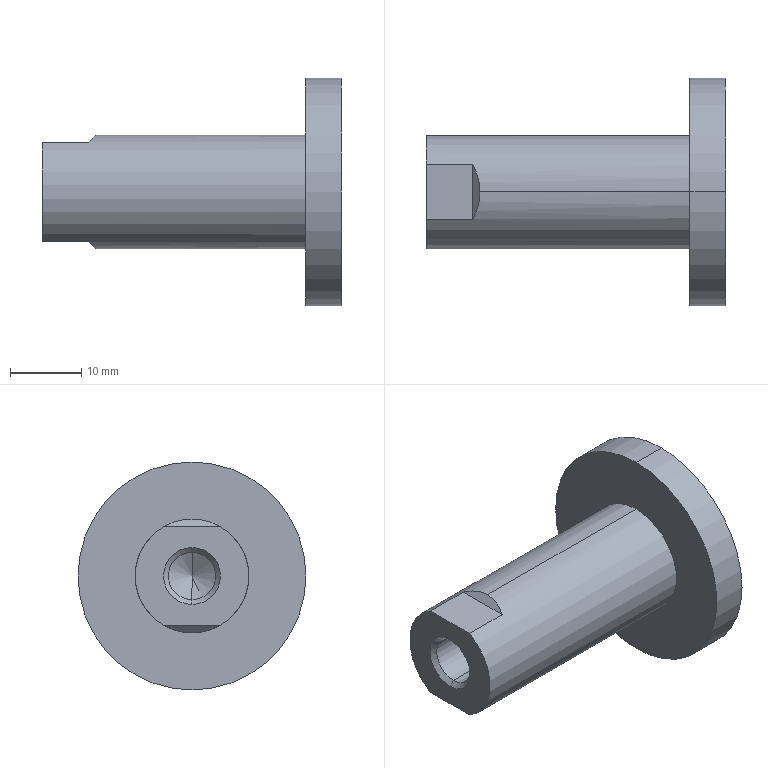Part | SolidWorks | features RefAxis 3, 3DProfileFeature 1, ICE 1, Revolution 1 | 1 solid | 17 faces | box 42 x 32 x 32 mm | volume 10910 mm3 | plane 7 | cylinder 6 | cone 4 | commonest cylinder face diameters 6.647 x2 16 x2 32 x2
STEP:
#1=CARTESIAN_POINT('',(35.,0.,16.));
#2=VERTEX_POINT('',#1);
#3=CARTESIAN_POINT('',(35.,0.,-16.));
#4=VERTEX_POINT('',#3);
#5=CARTESIAN_POINT('',(35.,0.,0.));
#6=DIRECTION('',(-1.,0.,0.));
#7=DIRECTION('',(0.,0.,1.));
#8=AXIS2_PLACEMENT_3D('',#5,#6,#7);
#9=CIRCLE('',#8,16.);
#10=EDGE_CURVE('',#2,#4,#9,.T.);
#11=ORIENTED_EDGE('',*,*,#10,.T.);
#12=CARTESIAN_POINT('',(30.,0.,-16.));
#13=VERTEX_POINT('',#12);
#14=CARTESIAN_POINT('',(35.,0.,-16.));
#15=DIRECTION('',(-1.,0.,0.));
#16=VECTOR('',#15,1000.);
#17=LINE('',#14,#16);
#18=EDGE_CURVE('',#4,#13,#17,.T.);
#19=ORIENTED_EDGE('',*,*,#18,.T.);
#20=CARTESIAN_POINT('',(30.,0.,16.));
#21=VERTEX_POINT('',#20);
#22=CARTESIAN_POINT('',(30.,0.,0.));
#23=DIRECTION('',(-1.,0.,0.));
#24=DIRECTION('',(0.,0.,1.));
#25=AXIS2_PLACEMENT_3D('',#22,#23,#24);
#26=CIRCLE('',#25,16.);
#27=EDGE_CURVE('',#21,#13,#26,.T.);
#28=ORIENTED_EDGE('',*,*,#27,.F.);
#29=CARTESIAN_POINT('',(35.,0.,16.));
#30=DIRECTION('',(-1.,0.,0.));
#31=VECTOR('',#30,1000.);
#32=LINE('',#29,#31);
#33=EDGE_CURVE('',#2,#21,#32,.T.);
#34=ORIENTED_EDGE('',*,*,#33,.F.);
#35=EDGE_LOOP('',(#11,#19,#28,#34));
#36=FACE_OUTER_BOUND('',#35,.T.);
#37=CARTESIAN_POINT('',(35.,0.,0.));
#38=DIRECTION('',(-1.,0.,0.));
#39=DIRECTION('',(0.,0.,1.));
#40=AXIS2_PLACEMENT_3D('',#37,#38,#39);
#41=CYLINDRICAL_SURFACE('',#40,16.);
#42=ADVANCED_FACE('',(#36),#41,.T.);
#43=CARTESIAN_POINT('',(30.,0.,8.));
#44=VERTEX_POINT('',#43);
#45=CARTESIAN_POINT('',(30.,0.,-8.));
#46=VERTEX_POINT('',#45);
#47=CARTESIAN_POINT('',(30.,0.,0.));
#48=DIRECTION('',(-1.,0.,0.));
#49=DIRECTION('',(0.,0.,1.));
#50=AXIS2_PLACEMENT_3D('',#47,#48,#49);
#51=CIRCLE('',#50,8.);
#52=EDGE_CURVE('',#44,#46,#51,.T.);
#53=ORIENTED_EDGE('',*,*,#52,.T.);
#54=CARTESIAN_POINT('',(0.5,0.,-8.));
#55=VERTEX_POINT('',#54);
#56=CARTESIAN_POINT('',(35.,0.,-8.));
#57=DIRECTION('',(-1.,0.,0.));
#58=VECTOR('',#57,1000.);
#59=LINE('',#56,#58);
#60=EDGE_CURVE('',#46,#55,#59,.T.);
#61=ORIENTED_EDGE('',*,*,#60,.T.);
#62=CARTESIAN_POINT('',(-0.5,3.873,-7.));
#63=VERTEX_POINT('',#62);
#64=CARTESIAN_POINT('',(0.5,0.,-8.));
#65=CARTESIAN_POINT('',(0.5,1.362,-8.));
#66=CARTESIAN_POINT('',(0.1595,2.681,-7.659));
#67=CARTESIAN_POINT('',(-0.5,3.873,-7.));
#68=(BOUNDED_CURVE()B_SPLINE_CURVE(3,(#64,#65,#66,#67),.UNSPECIFIED.,.F.,.F.)B_SPLINE_CURVE_WITH_KNOTS((4,4),(3.142,3.647),.UNSPECIFIED.)CURVE()GEOMETRIC_REPRESENTATION_ITEM()RATIONAL_B_SPLINE_CURVE((1.,0.9788,0.9788,1.))REPRESENTATION_ITEM(''));
#69=EDGE_CURVE('',#55,#63,#68,.T.);
#70=ORIENTED_EDGE('',*,*,#69,.T.);
#71=CARTESIAN_POINT('',(-7.,3.873,-7.));
#72=VERTEX_POINT('',#71);
#73=CARTESIAN_POINT('',(35.,3.873,-7.));
#74=DIRECTION('',(-1.,0.,0.));
#75=VECTOR('',#74,1000.);
#76=LINE('',#73,#75);
#77=EDGE_CURVE('',#63,#72,#76,.T.);
#78=ORIENTED_EDGE('',*,*,#77,.T.);
#79=CARTESIAN_POINT('',(-7.,3.873,7.));
#80=VERTEX_POINT('',#79);
#81=CARTESIAN_POINT('',(-7.,0.,0.));
#82=DIRECTION('',(-1.,0.,0.));
#83=DIRECTION('',(0.,0.,1.));
#84=AXIS2_PLACEMENT_3D('',#81,#82,#83);
#85=CIRCLE('',#84,8.);
#86=EDGE_CURVE('',#80,#72,#85,.T.);
#87=ORIENTED_EDGE('',*,*,#86,.F.);
#88=CARTESIAN_POINT('',(-0.5,3.873,7.));
#89=VERTEX_POINT('',#88);
#90=CARTESIAN_POINT('',(35.,3.873,7.));
#91=DIRECTION('',(1.,0.,0.));
#92=VECTOR('',#91,1000.);
#93=LINE('',#90,#92);
#94=EDGE_CURVE('',#80,#89,#93,.T.);
#95=ORIENTED_EDGE('',*,*,#94,.T.);
#96=CARTESIAN_POINT('',(0.5,0.,8.));
#97=VERTEX_POINT('',#96);
#98=CARTESIAN_POINT('',(-0.5,3.873,7.));
#99=CARTESIAN_POINT('',(0.1595,2.681,7.659));
#100=CARTESIAN_POINT('',(0.5,1.362,8.));
#101=CARTESIAN_POINT('',(0.5,0.,8.));
#102=(BOUNDED_CURVE()B_SPLINE_CURVE(3,(#98,#99,#100,#101),.UNSPECIFIED.,.F.,.T.)B_SPLINE_CURVE_WITH_KNOTS((4,4),(2.636,3.142),.UNSPECIFIED.)CURVE()GEOMETRIC_REPRESENTATION_ITEM()RATIONAL_B_SPLINE_CURVE((1.,0.9788,0.9788,1.))REPRESENTATION_ITEM(''));
#103=EDGE_CURVE('',#89,#97,#102,.T.);
#104=ORIENTED_EDGE('',*,*,#103,.T.);
#105=CARTESIAN_POINT('',(35.,0.,8.));
#106=DIRECTION('',(-1.,0.,0.));
#107=VECTOR('',#106,1000.);
#108=LINE('',#105,#107);
#109=EDGE_CURVE('',#44,#97,#108,.T.);
#110=ORIENTED_EDGE('',*,*,#109,.F.);
#111=EDGE_LOOP('',(#53,#61,#70,#78,#87,#95,#104,#110));
#112=FACE_OUTER_BOUND('',#111,.T.);
#113=CARTESIAN_POINT('',(35.,0.,0.));
#114=DIRECTION('',(-1.,0.,0.));
#115=DIRECTION('',(0.,0.,1.));
#116=AXIS2_PLACEMENT_3D('',#113,#114,#115);
#117=CYLINDRICAL_SURFACE('',#116,8.);
#118=ADVANCED_FACE('',(#112),#117,.T.);
#119=CARTESIAN_POINT('',(-6.324,0.,-3.324));
#120=VERTEX_POINT('',#119);
#121=CARTESIAN_POINT('',(-6.324,0.,3.324));
#122=VERTEX_POINT('',#121);
#123=CARTESIAN_POINT('',(-6.324,0.,0.));
#124=DIRECTION('',(-1.,0.,0.));
#125=DIRECTION('',(0.,0.,1.));
#126=AXIS2_PLACEMENT_3D('',#123,#124,#125);
#127=CIRCLE('',#126,3.324);
#128=EDGE_CURVE('',#120,#122,#127,.T.);
#129=ORIENTED_EDGE('',*,*,#128,.F.);
#130=CARTESIAN_POINT('',(-7.,0.,-4.));
#131=VERTEX_POINT('',#130);
#132=CARTESIAN_POINT('',(-7.,0.,-4.));
#133=DIRECTION('',(-0.7071,0.,-0.7071));
#134=VECTOR('',#133,1000.);
#135=LINE('',#132,#134);
#136=EDGE_CURVE('',#120,#131,#135,.T.);
#137=ORIENTED_EDGE('',*,*,#136,.T.);
#138=CARTESIAN_POINT('',(-7.,0.,4.));
#139=VERTEX_POINT('',#138);
#140=CARTESIAN_POINT('',(-7.,0.,0.));
#141=DIRECTION('',(-1.,0.,0.));
#142=DIRECTION('',(0.,0.,1.));
#143=AXIS2_PLACEMENT_3D('',#140,#141,#142);
#144=CIRCLE('',#143,4.);
#145=EDGE_CURVE('',#131,#139,#144,.T.);
#146=ORIENTED_EDGE('',*,*,#145,.T.);
#147=CARTESIAN_POINT('',(-7.,0.,4.));
#148=DIRECTION('',(-0.7071,0.,0.7071));
#149=VECTOR('',#148,1000.);
#150=LINE('',#147,#149);
#151=EDGE_CURVE('',#122,#139,#150,.T.);
#152=ORIENTED_EDGE('',*,*,#151,.F.);
#153=EDGE_LOOP('',(#129,#137,#146,#152));
#154=FACE_OUTER_BOUND('',#153,.T.);
#155=CARTESIAN_POINT('',(-7.,0.,0.));
#156=DIRECTION('',(-1.,0.,0.));
#157=DIRECTION('',(0.,0.,1.));
#158=AXIS2_PLACEMENT_3D('',#155,#156,#157);
#159=CONICAL_SURFACE('',#158,4.,0.7854);
#160=ADVANCED_FACE('',(#154),#159,.F.);
#161=CARTESIAN_POINT('',(6.,0.,-3.324));
#162=VERTEX_POINT('',#161);
#163=CARTESIAN_POINT('',(6.,0.,3.324));
#164=VERTEX_POINT('',#163);
#165=CARTESIAN_POINT('',(6.,0.,0.));
#166=DIRECTION('',(-1.,0.,0.));
#167=DIRECTION('',(0.,0.,1.));
#168=AXIS2_PLACEMENT_3D('',#165,#166,#167);
#169=CIRCLE('',#168,3.324);
#170=EDGE_CURVE('',#162,#164,#169,.T.);
#171=ORIENTED_EDGE('',*,*,#170,.F.);
#172=CARTESIAN_POINT('',(35.,0.,-3.324));
#173=DIRECTION('',(-1.,0.,0.));
#174=VECTOR('',#173,1000.);
#175=LINE('',#172,#174);
#176=EDGE_CURVE('',#162,#120,#175,.T.);
#177=ORIENTED_EDGE('',*,*,#176,.T.);
#178=ORIENTED_EDGE('',*,*,#128,.T.);
#179=CARTESIAN_POINT('',(35.,0.,3.324));
#180=DIRECTION('',(-1.,0.,0.));
#181=VECTOR('',#180,1000.);
#182=LINE('',#179,#181);
#183=EDGE_CURVE('',#164,#122,#182,.T.);
#184=ORIENTED_EDGE('',*,*,#183,.F.);
#185=EDGE_LOOP('',(#171,#177,#178,#184));
#186=FACE_OUTER_BOUND('',#185,.T.);
#187=CARTESIAN_POINT('',(35.,0.,0.));
#188=DIRECTION('',(-1.,0.,0.));
#189=DIRECTION('',(0.,0.,1.));
#190=AXIS2_PLACEMENT_3D('',#187,#188,#189);
#191=CYLINDRICAL_SURFACE('',#190,3.324);
#192=ADVANCED_FACE('',(#186),#191,.F.);
#193=CARTESIAN_POINT('',(7.919,0.,0.));
#194=VERTEX_POINT('',#193);
#195=CARTESIAN_POINT('',(6.,0.,3.324));
#196=DIRECTION('',(-0.5,0.,0.866));
#197=VECTOR('',#196,1000.);
#198=LINE('',#195,#197);
#199=EDGE_CURVE('',#194,#164,#198,.T.);
#200=ORIENTED_EDGE('',*,*,#199,.F.);
#201=CARTESIAN_POINT('',(6.,0.,-3.324));
#202=DIRECTION('',(-0.5,0.,-0.866));
#203=VECTOR('',#202,1000.);
#204=LINE('',#201,#203);
#205=EDGE_CURVE('',#194,#162,#204,.T.);
#206=ORIENTED_EDGE('',*,*,#205,.T.);
#207=ORIENTED_EDGE('',*,*,#170,.T.);
#208=EDGE_LOOP('',(#200,#206,#207));
#209=FACE_OUTER_BOUND('',#208,.T.);
#210=CARTESIAN_POINT('',(6.,0.,0.));
#211=DIRECTION('',(-1.,0.,0.));
#212=DIRECTION('',(0.,0.,1.));
#213=AXIS2_PLACEMENT_3D('',#210,#211,#212);
#214=CONICAL_SURFACE('',#213,3.324,1.047);
#215=ADVANCED_FACE('',(#209),#214,.F.);
#216=ORIENTED_EDGE('',*,*,#205,.F.);
#217=ORIENTED_EDGE('',*,*,#199,.T.);
#218=CARTESIAN_POINT('',(6.,0.,0.));
#219=DIRECTION('',(-1.,0.,0.));
#220=DIRECTION('',(0.,0.,1.));
#221=AXIS2_PLACEMENT_3D('',#218,#219,#220);
#222=CIRCLE('',#221,3.324);
#223=EDGE_CURVE('',#164,#162,#222,.T.);
#224=ORIENTED_EDGE('',*,*,#223,.T.);
#225=EDGE_LOOP('',(#216,#217,#224));
#226=FACE_OUTER_BOUND('',#225,.T.);
#227=CARTESIAN_POINT('',(6.,0.,0.));
#228=DIRECTION('',(-1.,0.,0.));
#229=DIRECTION('',(0.,0.,1.));
#230=AXIS2_PLACEMENT_3D('',#227,#228,#229);
#231=CONICAL_SURFACE('',#230,3.324,1.047);
#232=ADVANCED_FACE('',(#226),#231,.F.);
#233=ORIENTED_EDGE('',*,*,#176,.F.);
#234=ORIENTED_EDGE('',*,*,#223,.F.);
#235=ORIENTED_EDGE('',*,*,#183,.T.);
#236=CARTESIAN_POINT('',(-6.324,0.,0.));
#237=DIRECTION('',(-1.,0.,0.));
#238=DIRECTION('',(0.,0.,1.));
#239=AXIS2_PLACEMENT_3D('',#236,#237,#238);
#240=CIRCLE('',#239,3.324);
#241=EDGE_CURVE('',#122,#120,#240,.T.);
#242=ORIENTED_EDGE('',*,*,#241,.T.);
#243=EDGE_LOOP('',(#233,#234,#235,#242));
#244=FACE_OUTER_BOUND('',#243,.T.);
#245=CARTESIAN_POINT('',(35.,0.,0.));
#246=DIRECTION('',(-1.,0.,0.));
#247=DIRECTION('',(0.,0.,1.));
#248=AXIS2_PLACEMENT_3D('',#245,#246,#247);
#249=CYLINDRICAL_SURFACE('',#248,3.324);
#250=ADVANCED_FACE('',(#244),#249,.F.);
#251=ORIENTED_EDGE('',*,*,#136,.F.);
#252=ORIENTED_EDGE('',*,*,#241,.F.);
#253=ORIENTED_EDGE('',*,*,#151,.T.);
#254=CARTESIAN_POINT('',(-7.,0.,0.));
#255=DIRECTION('',(-1.,0.,0.));
#256=DIRECTION('',(0.,0.,1.));
#257=AXIS2_PLACEMENT_3D('',#254,#255,#256);
#258=CIRCLE('',#257,4.);
#259=EDGE_CURVE('',#139,#131,#258,.T.);
#260=ORIENTED_EDGE('',*,*,#259,.T.);
#261=EDGE_LOOP('',(#251,#252,#253,#260));
#262=FACE_OUTER_BOUND('',#261,.T.);
#263=CARTESIAN_POINT('',(-7.,0.,0.));
#264=DIRECTION('',(-1.,0.,0.));
#265=DIRECTION('',(0.,0.,1.));
#266=AXIS2_PLACEMENT_3D('',#263,#264,#265);
#267=CONICAL_SURFACE('',#266,4.,0.7854);
#268=ADVANCED_FACE('',(#262),#267,.F.);
#269=ORIENTED_EDGE('',*,*,#259,.F.);
#270=ORIENTED_EDGE('',*,*,#145,.F.);
#271=EDGE_LOOP('',(#269,#270));
#272=FACE_BOUND('',#271,.T.);
#273=ORIENTED_EDGE('',*,*,#86,.T.);
#274=CARTESIAN_POINT('',(-7.,-3.873,-7.));
#275=VERTEX_POINT('',#274);
#276=CARTESIAN_POINT('',(-7.,-16.,-7.));
#277=DIRECTION('',(0.,1.,0.));
#278=VECTOR('',#277,1000.);
#279=LINE('',#276,#278);
#280=EDGE_CURVE('',#275,#72,#279,.T.);
#281=ORIENTED_EDGE('',*,*,#280,.F.);
#282=CARTESIAN_POINT('',(-7.,-3.873,7.));
#283=VERTEX_POINT('',#282);
#284=CARTESIAN_POINT('',(-7.,0.,0.));
#285=DIRECTION('',(-1.,0.,0.));
#286=DIRECTION('',(0.,0.,1.));
#287=AXIS2_PLACEMENT_3D('',#284,#285,#286);
#288=CIRCLE('',#287,8.);
#289=EDGE_CURVE('',#275,#283,#288,.T.);
#290=ORIENTED_EDGE('',*,*,#289,.T.);
#291=CARTESIAN_POINT('',(-7.,-16.,7.));
#292=DIRECTION('',(0.,1.,0.));
#293=VECTOR('',#292,1000.);
#294=LINE('',#291,#293);
#295=EDGE_CURVE('',#283,#80,#294,.T.);
#296=ORIENTED_EDGE('',*,*,#295,.T.);
#297=EDGE_LOOP('',(#273,#281,#290,#296));
#298=FACE_OUTER_BOUND('',#297,.T.);
#299=CARTESIAN_POINT('',(-7.,4.,0.));
#300=DIRECTION('',(1.,0.,0.));
#301=DIRECTION('',(0.,0.,-1.));
#302=AXIS2_PLACEMENT_3D('',#299,#300,#301);
#303=PLANE('',#302);
#304=ADVANCED_FACE('',(#272,#298),#303,.F.);
#305=ORIENTED_EDGE('',*,*,#60,.F.);
#306=CARTESIAN_POINT('',(30.,0.,0.));
#307=DIRECTION('',(-1.,0.,0.));
#308=DIRECTION('',(0.,0.,1.));
#309=AXIS2_PLACEMENT_3D('',#306,#307,#308);
#310=CIRCLE('',#309,8.);
#311=EDGE_CURVE('',#46,#44,#310,.T.);
#312=ORIENTED_EDGE('',*,*,#311,.T.);
#313=ORIENTED_EDGE('',*,*,#109,.T.);
#314=CARTESIAN_POINT('',(-0.5,-3.873,7.));
#315=VERTEX_POINT('',#314);
#316=CARTESIAN_POINT('',(0.5,0.,8.));
#317=CARTESIAN_POINT('',(0.5,-1.362,8.));
#318=CARTESIAN_POINT('',(0.1595,-2.681,7.659));
#319=CARTESIAN_POINT('',(-0.5,-3.873,7.));
#320=(BOUNDED_CURVE()B_SPLINE_CURVE(3,(#316,#317,#318,#319),.UNSPECIFIED.,.F.,.F.)B_SPLINE_CURVE_WITH_KNOTS((4,4),(3.142,3.647),.UNSPECIFIED.)CURVE()GEOMETRIC_REPRESENTATION_ITEM()RATIONAL_B_SPLINE_CURVE((1.,0.9788,0.9788,1.))REPRESENTATION_ITEM(''));
#321=EDGE_CURVE('',#97,#315,#320,.T.);
#322=ORIENTED_EDGE('',*,*,#321,.T.);
#323=CARTESIAN_POINT('',(35.,-3.873,7.));
#324=DIRECTION('',(-1.,0.,0.));
#325=VECTOR('',#324,1000.);
#326=LINE('',#323,#325);
#327=EDGE_CURVE('',#315,#283,#326,.T.);
#328=ORIENTED_EDGE('',*,*,#327,.T.);
#329=ORIENTED_EDGE('',*,*,#289,.F.);
#330=CARTESIAN_POINT('',(-0.5,-3.873,-7.));
#331=VERTEX_POINT('',#330);
#332=CARTESIAN_POINT('',(35.,-3.873,-7.));
#333=DIRECTION('',(1.,0.,0.));
#334=VECTOR('',#333,1000.);
#335=LINE('',#332,#334);
#336=EDGE_CURVE('',#275,#331,#335,.T.);
#337=ORIENTED_EDGE('',*,*,#336,.T.);
#338=CARTESIAN_POINT('',(-0.5,-3.873,-7.));
#339=CARTESIAN_POINT('',(0.1595,-2.681,-7.659));
#340=CARTESIAN_POINT('',(0.5,-1.362,-8.));
#341=CARTESIAN_POINT('',(0.5,0.,-8.));
#342=(BOUNDED_CURVE()B_SPLINE_CURVE(3,(#338,#339,#340,#341),.UNSPECIFIED.,.F.,.F.)B_SPLINE_CURVE_WITH_KNOTS((4,4),(2.636,3.142),.UNSPECIFIED.)CURVE()GEOMETRIC_REPRESENTATION_ITEM()RATIONAL_B_SPLINE_CURVE((1.,0.9788,0.9788,1.))REPRESENTATION_ITEM(''));
#343=EDGE_CURVE('',#331,#55,#342,.T.);
#344=ORIENTED_EDGE('',*,*,#343,.T.);
#345=EDGE_LOOP('',(#305,#312,#313,#322,#328,#329,#337,#344));
#346=FACE_OUTER_BOUND('',#345,.T.);
#347=CARTESIAN_POINT('',(35.,0.,0.));
#348=DIRECTION('',(-1.,0.,0.));
#349=DIRECTION('',(0.,0.,1.));
#350=AXIS2_PLACEMENT_3D('',#347,#348,#349);
#351=CYLINDRICAL_SURFACE('',#350,8.);
#352=ADVANCED_FACE('',(#346),#351,.T.);
#353=ORIENTED_EDGE('',*,*,#52,.F.);
#354=ORIENTED_EDGE('',*,*,#311,.F.);
#355=EDGE_LOOP('',(#353,#354));
#356=FACE_BOUND('',#355,.T.);
#357=ORIENTED_EDGE('',*,*,#27,.T.);
#358=CARTESIAN_POINT('',(30.,0.,0.));
#359=DIRECTION('',(-1.,0.,0.));
#360=DIRECTION('',(0.,0.,1.));
#361=AXIS2_PLACEMENT_3D('',#358,#359,#360);
#362=CIRCLE('',#361,16.);
#363=EDGE_CURVE('',#13,#21,#362,.T.);
#364=ORIENTED_EDGE('',*,*,#363,.T.);
#365=EDGE_LOOP('',(#357,#364));
#366=FACE_OUTER_BOUND('',#365,.T.);
#367=CARTESIAN_POINT('',(30.,8.,0.));
#368=DIRECTION('',(1.,0.,0.));
#369=DIRECTION('',(0.,0.,-1.));
#370=AXIS2_PLACEMENT_3D('',#367,#368,#369);
#371=PLANE('',#370);
#372=ADVANCED_FACE('',(#356,#366),#371,.F.);
#373=ORIENTED_EDGE('',*,*,#18,.F.);
#374=CARTESIAN_POINT('',(35.,0.,0.));
#375=DIRECTION('',(-1.,0.,0.));
#376=DIRECTION('',(0.,0.,1.));
#377=AXIS2_PLACEMENT_3D('',#374,#375,#376);
#378=CIRCLE('',#377,16.);
#379=EDGE_CURVE('',#4,#2,#378,.T.);
#380=ORIENTED_EDGE('',*,*,#379,.T.);
#381=ORIENTED_EDGE('',*,*,#33,.T.);
#382=ORIENTED_EDGE('',*,*,#363,.F.);
#383=EDGE_LOOP('',(#373,#380,#381,#382));
#384=FACE_OUTER_BOUND('',#383,.T.);
#385=CARTESIAN_POINT('',(35.,0.,0.));
#386=DIRECTION('',(-1.,0.,0.));
#387=DIRECTION('',(0.,0.,1.));
#388=AXIS2_PLACEMENT_3D('',#385,#386,#387);
#389=CYLINDRICAL_SURFACE('',#388,16.);
#390=ADVANCED_FACE('',(#384),#389,.T.);
#391=ORIENTED_EDGE('',*,*,#10,.F.);
#392=ORIENTED_EDGE('',*,*,#379,.F.);
#393=EDGE_LOOP('',(#391,#392));
#394=FACE_OUTER_BOUND('',#393,.T.);
#395=CARTESIAN_POINT('',(35.,16.,0.));
#396=DIRECTION('',(-1.,0.,0.));
#397=DIRECTION('',(0.,0.,1.));
#398=AXIS2_PLACEMENT_3D('',#395,#396,#397);
#399=PLANE('',#398);
#400=ADVANCED_FACE('',(#394),#399,.F.);
#401=CARTESIAN_POINT('',(-0.5,-16.,7.));
#402=DIRECTION('',(0.,1.,0.));
#403=VECTOR('',#402,1000.);
#404=LINE('',#401,#403);
#405=EDGE_CURVE('',#315,#89,#404,.T.);
#406=ORIENTED_EDGE('',*,*,#405,.F.);
#407=ORIENTED_EDGE('',*,*,#321,.F.);
#408=ORIENTED_EDGE('',*,*,#103,.F.);
#409=EDGE_LOOP('',(#406,#407,#408));
#410=FACE_OUTER_BOUND('',#409,.T.);
#411=CARTESIAN_POINT('',(4.5,-16.,12.));
#412=DIRECTION('',(0.7071,0.,-0.7071));
#413=DIRECTION('',(-0.7071,0.,-0.7071));
#414=AXIS2_PLACEMENT_3D('',#411,#412,#413);
#415=PLANE('',#414);
#416=ADVANCED_FACE('',(#410),#415,.F.);
#417=ORIENTED_EDGE('',*,*,#405,.T.);
#418=ORIENTED_EDGE('',*,*,#94,.F.);
#419=ORIENTED_EDGE('',*,*,#295,.F.);
#420=ORIENTED_EDGE('',*,*,#327,.F.);
#421=EDGE_LOOP('',(#417,#418,#419,#420));
#422=FACE_OUTER_BOUND('',#421,.T.);
#423=CARTESIAN_POINT('',(-0.5,-16.,7.));
#424=DIRECTION('',(0.,0.,-1.));
#425=DIRECTION('',(-1.,0.,0.));
#426=AXIS2_PLACEMENT_3D('',#423,#424,#425);
#427=PLANE('',#426);
#428=ADVANCED_FACE('',(#422),#427,.F.);
#429=CARTESIAN_POINT('',(-0.5,-16.,-7.));
#430=DIRECTION('',(0.,1.,0.));
#431=VECTOR('',#430,1000.);
#432=LINE('',#429,#431);
#433=EDGE_CURVE('',#331,#63,#432,.T.);
#434=ORIENTED_EDGE('',*,*,#433,.T.);
#435=ORIENTED_EDGE('',*,*,#69,.F.);
#436=ORIENTED_EDGE('',*,*,#343,.F.);
#437=EDGE_LOOP('',(#434,#435,#436));
#438=FACE_OUTER_BOUND('',#437,.T.);
#439=CARTESIAN_POINT('',(-0.5,-16.,-7.));
#440=DIRECTION('',(0.7071,0.,0.7071));
#441=DIRECTION('',(0.7071,0.,-0.7071));
#442=AXIS2_PLACEMENT_3D('',#439,#440,#441);
#443=PLANE('',#442);
#444=ADVANCED_FACE('',(#438),#443,.F.);
#445=ORIENTED_EDGE('',*,*,#433,.F.);
#446=ORIENTED_EDGE('',*,*,#336,.F.);
#447=ORIENTED_EDGE('',*,*,#280,.T.);
#448=ORIENTED_EDGE('',*,*,#77,.F.);
#449=EDGE_LOOP('',(#445,#446,#447,#448));
#450=FACE_OUTER_BOUND('',#449,.T.);
#451=CARTESIAN_POINT('',(-7.,-16.,-7.));
#452=DIRECTION('',(0.,0.,1.));
#453=DIRECTION('',(1.,0.,0.));
#454=AXIS2_PLACEMENT_3D('',#451,#452,#453);
#455=PLANE('',#454);
#456=ADVANCED_FACE('',(#450),#455,.F.);
#457=CLOSED_SHELL('',(#42,#118,#160,#192,#215,#232,#250,#268,#304,#352,#372,#390,#400,#416,#428,#444,#456));
#458=MANIFOLD_SOLID_BREP('',#457);
#459=CARTESIAN_POINT('',(0.,0.,0.));
#460=DIRECTION('',(0.,0.,1.));
#461=DIRECTION('',(1.,0.,0.));
#462=AXIS2_PLACEMENT_3D('',#459,#460,#461);
#463=(LENGTH_UNIT()NAMED_UNIT(*)SI_UNIT(.MILLI.,.METRE.));
#464=UNCERTAINTY_MEASURE_WITH_UNIT(LENGTH_MEASURE(0.00001),#463,'','');
#465=(NAMED_UNIT(*)PLANE_ANGLE_UNIT()SI_UNIT($,.RADIAN.));
#466=(NAMED_UNIT(*)SI_UNIT($,.STERADIAN.)SOLID_ANGLE_UNIT());
#467=(GEOMETRIC_REPRESENTATION_CONTEXT(3)GLOBAL_UNCERTAINTY_ASSIGNED_CONTEXT((#464))GLOBAL_UNIT_ASSIGNED_CONTEXT((#463,#465,#466))REPRESENTATION_CONTEXT('',''));
#468=ADVANCED_BREP_SHAPE_REPRESENTATION('',(#458,#462),#467);